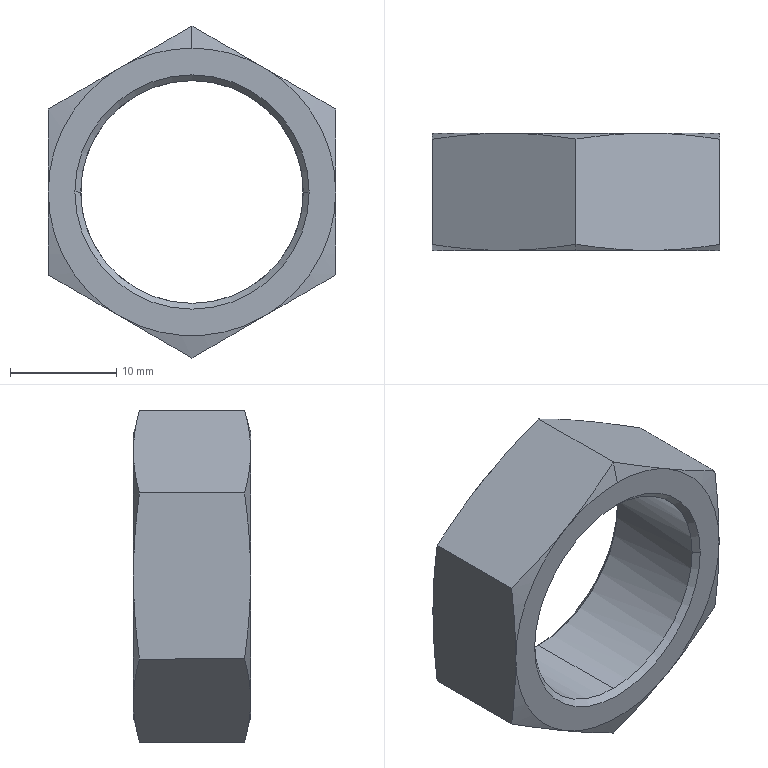Part | STEP file | 3 | 1 solid | 27 faces | box 27 x 11 x 31.177 mm | volume 3125 mm3 | cone 17 | plane 8 | cylinder 2 | commonest cylinder face diameters 20.917 x2
STEP:
#1=CARTESIAN_POINT('',(0.,10.541,-10.459));
#2=VERTEX_POINT('',#1);
#3=CARTESIAN_POINT('',(-10.459,10.541,0.));
#4=VERTEX_POINT('',#3);
#5=CARTESIAN_POINT('',(0.,10.541,0.));
#6=DIRECTION('',(0.,1.,0.));
#7=DIRECTION('',(0.,0.,1.));
#8=AXIS2_PLACEMENT_3D('',#5,#6,#7);
#9=CIRCLE('',#8,10.459);
#10=EDGE_CURVE('',#2,#4,#9,.T.);
#11=ORIENTED_EDGE('',*,*,#10,.F.);
#12=CARTESIAN_POINT('',(0.,20.459,-10.459));
#13=VERTEX_POINT('',#12);
#14=CARTESIAN_POINT('',(0.,15.5,-10.459));
#15=DIRECTION('',(0.,1.,0.));
#16=VECTOR('',#15,1000.);
#17=LINE('',#14,#16);
#18=EDGE_CURVE('',#2,#13,#17,.T.);
#19=ORIENTED_EDGE('',*,*,#18,.T.);
#20=CARTESIAN_POINT('',(0.,20.459,10.459));
#21=VERTEX_POINT('',#20);
#22=CARTESIAN_POINT('',(0.,20.459,0.));
#23=DIRECTION('',(0.,-1.,0.));
#24=DIRECTION('',(0.,0.,1.));
#25=AXIS2_PLACEMENT_3D('',#22,#23,#24);
#26=CIRCLE('',#25,10.459);
#27=EDGE_CURVE('',#21,#13,#26,.T.);
#28=ORIENTED_EDGE('',*,*,#27,.F.);
#29=CARTESIAN_POINT('',(0.,10.541,10.459));
#30=VERTEX_POINT('',#29);
#31=CARTESIAN_POINT('',(0.,15.5,10.459));
#32=DIRECTION('',(0.,1.,0.));
#33=VECTOR('',#32,1000.);
#34=LINE('',#31,#33);
#35=EDGE_CURVE('',#30,#21,#34,.T.);
#36=ORIENTED_EDGE('',*,*,#35,.F.);
#37=CARTESIAN_POINT('',(0.,10.541,0.));
#38=DIRECTION('',(0.,1.,0.));
#39=DIRECTION('',(0.,0.,1.));
#40=AXIS2_PLACEMENT_3D('',#37,#38,#39);
#41=CIRCLE('',#40,10.459);
#42=EDGE_CURVE('',#4,#30,#41,.T.);
#43=ORIENTED_EDGE('',*,*,#42,.F.);
#44=EDGE_LOOP('',(#11,#19,#28,#36,#43));
#45=FACE_OUTER_BOUND('',#44,.T.);
#46=CARTESIAN_POINT('',(0.,15.5,0.));
#47=DIRECTION('',(0.,1.,0.));
#48=DIRECTION('',(0.,0.,1.));
#49=AXIS2_PLACEMENT_3D('',#46,#47,#48);
#50=CYLINDRICAL_SURFACE('',#49,10.459);
#51=ADVANCED_FACE('',(#45),#50,.F.);
#52=CARTESIAN_POINT('',(10.459,10.541,0.));
#53=VERTEX_POINT('',#52);
#54=CARTESIAN_POINT('',(0.,10.541,0.));
#55=DIRECTION('',(0.,1.,0.));
#56=DIRECTION('',(0.,0.,1.));
#57=AXIS2_PLACEMENT_3D('',#54,#55,#56);
#58=CIRCLE('',#57,10.459);
#59=EDGE_CURVE('',#53,#2,#58,.T.);
#60=ORIENTED_EDGE('',*,*,#59,.T.);
#61=ORIENTED_EDGE('',*,*,#10,.T.);
#62=CARTESIAN_POINT('',(-11.,10.,0.));
#63=VERTEX_POINT('',#62);
#64=CARTESIAN_POINT('',(-11.,10.,0.));
#65=DIRECTION('',(-0.7071,-0.7071,0.));
#66=VECTOR('',#65,1000.);
#67=LINE('',#64,#66);
#68=EDGE_CURVE('',#4,#63,#67,.T.);
#69=ORIENTED_EDGE('',*,*,#68,.T.);
#70=CARTESIAN_POINT('',(11.,10.,0.));
#71=VERTEX_POINT('',#70);
#72=CARTESIAN_POINT('',(0.,10.,0.));
#73=DIRECTION('',(0.,1.,0.));
#74=DIRECTION('',(1.,0.,0.));
#75=AXIS2_PLACEMENT_3D('',#72,#73,#74);
#76=CIRCLE('',#75,11.);
#77=EDGE_CURVE('',#71,#63,#76,.T.);
#78=ORIENTED_EDGE('',*,*,#77,.F.);
#79=CARTESIAN_POINT('',(11.,10.,0.));
#80=DIRECTION('',(0.7071,-0.7071,0.));
#81=VECTOR('',#80,1000.);
#82=LINE('',#79,#81);
#83=EDGE_CURVE('',#53,#71,#82,.T.);
#84=ORIENTED_EDGE('',*,*,#83,.F.);
#85=EDGE_LOOP('',(#60,#61,#69,#78,#84));
#86=FACE_OUTER_BOUND('',#85,.T.);
#87=CARTESIAN_POINT('',(0.,10.,0.));
#88=DIRECTION('',(0.,-1.,0.));
#89=DIRECTION('',(1.,0.,0.));
#90=AXIS2_PLACEMENT_3D('',#87,#88,#89);
#91=CONICAL_SURFACE('',#90,11.,0.7854);
#92=ADVANCED_FACE('',(#86),#91,.F.);
#93=ORIENTED_EDGE('',*,*,#27,.T.);
#94=CARTESIAN_POINT('',(0.,21.,-11.));
#95=VERTEX_POINT('',#94);
#96=CARTESIAN_POINT('',(0.,21.,-11.));
#97=DIRECTION('',(0.,0.7071,-0.7071));
#98=VECTOR('',#97,1000.);
#99=LINE('',#96,#98);
#100=EDGE_CURVE('',#13,#95,#99,.T.);
#101=ORIENTED_EDGE('',*,*,#100,.T.);
#102=CARTESIAN_POINT('',(0.,21.,11.));
#103=VERTEX_POINT('',#102);
#104=CARTESIAN_POINT('',(0.,21.,0.));
#105=DIRECTION('',(0.,-1.,0.));
#106=DIRECTION('',(0.,0.,1.));
#107=AXIS2_PLACEMENT_3D('',#104,#105,#106);
#108=CIRCLE('',#107,11.);
#109=EDGE_CURVE('',#103,#95,#108,.T.);
#110=ORIENTED_EDGE('',*,*,#109,.F.);
#111=CARTESIAN_POINT('',(0.,21.,11.));
#112=DIRECTION('',(0.,0.7071,0.7071));
#113=VECTOR('',#112,1000.);
#114=LINE('',#111,#113);
#115=EDGE_CURVE('',#21,#103,#114,.T.);
#116=ORIENTED_EDGE('',*,*,#115,.F.);
#117=EDGE_LOOP('',(#93,#101,#110,#116));
#118=FACE_OUTER_BOUND('',#117,.T.);
#119=CARTESIAN_POINT('',(0.,21.,0.));
#120=DIRECTION('',(0.,1.,0.));
#121=DIRECTION('',(0.,0.,1.));
#122=AXIS2_PLACEMENT_3D('',#119,#120,#121);
#123=CONICAL_SURFACE('',#122,11.,0.7854);
#124=ADVANCED_FACE('',(#118),#123,.F.);
#125=CARTESIAN_POINT('',(0.,10.,13.5));
#126=VERTEX_POINT('',#125);
#127=CARTESIAN_POINT('',(-6.75,10.,11.691));
#128=VERTEX_POINT('',#127);
#129=CARTESIAN_POINT('',(0.,10.,0.));
#130=DIRECTION('',(0.,-1.,0.));
#131=DIRECTION('',(0.,0.,1.));
#132=AXIS2_PLACEMENT_3D('',#129,#130,#131);
#133=CIRCLE('',#132,13.5);
#134=EDGE_CURVE('',#126,#128,#133,.T.);
#135=ORIENTED_EDGE('',*,*,#134,.F.);
#136=CARTESIAN_POINT('',(0.,10.56,15.588));
#137=VERTEX_POINT('',#136);
#138=CARTESIAN_POINT('',(0.,10.563,15.601));
#139=DIRECTION('',(0.,0.2588,0.9659));
#140=VECTOR('',#139,1000.);
#141=LINE('',#138,#140);
#142=EDGE_CURVE('',#126,#137,#141,.T.);
#143=ORIENTED_EDGE('',*,*,#142,.T.);
#144=CARTESIAN_POINT('',(0.,10.56,15.588));
#145=CARTESIAN_POINT('',(-1.12,10.386,14.942));
#146=CARTESIAN_POINT('',(-2.242,10.245,14.294));
#147=CARTESIAN_POINT('',(-4.492,10.052,12.995));
#148=CARTESIAN_POINT('',(-5.619,10.,12.344));
#149=CARTESIAN_POINT('',(-6.75,10.,11.691));
#150=B_SPLINE_CURVE_WITH_KNOTS('',3,(#144,#145,#146,#147,#148,#149),.UNSPECIFIED.,.F.,.F.,(4,2,4),(0.,0.003907,0.007814),.UNSPECIFIED.);
#151=EDGE_CURVE('',#137,#128,#150,.T.);
#152=ORIENTED_EDGE('',*,*,#151,.T.);
#153=EDGE_LOOP('',(#135,#143,#152));
#154=FACE_OUTER_BOUND('',#153,.T.);
#155=CARTESIAN_POINT('',(0.,10.563,0.));
#156=DIRECTION('',(0.,1.,0.));
#157=DIRECTION('',(0.,0.,1.));
#158=AXIS2_PLACEMENT_3D('',#155,#156,#157);
#159=CONICAL_SURFACE('',#158,15.601,1.309);
#160=ADVANCED_FACE('',(#154),#159,.T.);
#161=ORIENTED_EDGE('',*,*,#18,.F.);
#162=ORIENTED_EDGE('',*,*,#59,.F.);
#163=CARTESIAN_POINT('',(0.,10.541,0.));
#164=DIRECTION('',(0.,1.,0.));
#165=DIRECTION('',(0.,0.,1.));
#166=AXIS2_PLACEMENT_3D('',#163,#164,#165);
#167=CIRCLE('',#166,10.459);
#168=EDGE_CURVE('',#30,#53,#167,.T.);
#169=ORIENTED_EDGE('',*,*,#168,.F.);
#170=ORIENTED_EDGE('',*,*,#35,.T.);
#171=CARTESIAN_POINT('',(0.,20.459,0.));
#172=DIRECTION('',(0.,-1.,0.));
#173=DIRECTION('',(0.,0.,1.));
#174=AXIS2_PLACEMENT_3D('',#171,#172,#173);
#175=CIRCLE('',#174,10.459);
#176=EDGE_CURVE('',#13,#21,#175,.T.);
#177=ORIENTED_EDGE('',*,*,#176,.F.);
#178=EDGE_LOOP('',(#161,#162,#169,#170,#177));
#179=FACE_OUTER_BOUND('',#178,.T.);
#180=CARTESIAN_POINT('',(0.,15.5,0.));
#181=DIRECTION('',(0.,1.,0.));
#182=DIRECTION('',(0.,0.,1.));
#183=AXIS2_PLACEMENT_3D('',#180,#181,#182);
#184=CYLINDRICAL_SURFACE('',#183,10.459);
#185=ADVANCED_FACE('',(#179),#184,.F.);
#186=ORIENTED_EDGE('',*,*,#68,.F.);
#187=ORIENTED_EDGE('',*,*,#42,.T.);
#188=ORIENTED_EDGE('',*,*,#168,.T.);
#189=ORIENTED_EDGE('',*,*,#83,.T.);
#190=CARTESIAN_POINT('',(0.,10.,0.));
#191=DIRECTION('',(0.,1.,0.));
#192=DIRECTION('',(1.,0.,0.));
#193=AXIS2_PLACEMENT_3D('',#190,#191,#192);
#194=CIRCLE('',#193,11.);
#195=EDGE_CURVE('',#63,#71,#194,.T.);
#196=ORIENTED_EDGE('',*,*,#195,.F.);
#197=EDGE_LOOP('',(#186,#187,#188,#189,#196));
#198=FACE_OUTER_BOUND('',#197,.T.);
#199=CARTESIAN_POINT('',(0.,10.,0.));
#200=DIRECTION('',(0.,-1.,0.));
#201=DIRECTION('',(1.,0.,0.));
#202=AXIS2_PLACEMENT_3D('',#199,#200,#201);
#203=CONICAL_SURFACE('',#202,11.,0.7854);
#204=ADVANCED_FACE('',(#198),#203,.F.);
#205=ORIENTED_EDGE('',*,*,#100,.F.);
#206=ORIENTED_EDGE('',*,*,#176,.T.);
#207=ORIENTED_EDGE('',*,*,#115,.T.);
#208=CARTESIAN_POINT('',(0.,21.,0.));
#209=DIRECTION('',(0.,-1.,0.));
#210=DIRECTION('',(0.,0.,1.));
#211=AXIS2_PLACEMENT_3D('',#208,#209,#210);
#212=CIRCLE('',#211,11.);
#213=EDGE_CURVE('',#95,#103,#212,.T.);
#214=ORIENTED_EDGE('',*,*,#213,.F.);
#215=EDGE_LOOP('',(#205,#206,#207,#214));
#216=FACE_OUTER_BOUND('',#215,.T.);
#217=CARTESIAN_POINT('',(0.,21.,0.));
#218=DIRECTION('',(0.,1.,0.));
#219=DIRECTION('',(0.,0.,1.));
#220=AXIS2_PLACEMENT_3D('',#217,#218,#219);
#221=CONICAL_SURFACE('',#220,11.,0.7854);
#222=ADVANCED_FACE('',(#216),#221,.F.);
#223=CARTESIAN_POINT('',(-13.5,10.,0.));
#224=VERTEX_POINT('',#223);
#225=CARTESIAN_POINT('',(0.,10.,0.));
#226=DIRECTION('',(0.,-1.,0.));
#227=DIRECTION('',(0.,0.,1.));
#228=AXIS2_PLACEMENT_3D('',#225,#226,#227);
#229=CIRCLE('',#228,13.5);
#230=EDGE_CURVE('',#128,#224,#229,.T.);
#231=ORIENTED_EDGE('',*,*,#230,.T.);
#232=CARTESIAN_POINT('',(-6.75,10.,-11.691));
#233=VERTEX_POINT('',#232);
#234=CARTESIAN_POINT('',(0.,10.,0.));
#235=DIRECTION('',(0.,-1.,0.));
#236=DIRECTION('',(0.,0.,1.));
#237=AXIS2_PLACEMENT_3D('',#234,#235,#236);
#238=CIRCLE('',#237,13.5);
#239=EDGE_CURVE('',#224,#233,#238,.T.);
#240=ORIENTED_EDGE('',*,*,#239,.T.);
#241=CARTESIAN_POINT('',(6.75,10.,-11.691));
#242=VERTEX_POINT('',#241);
#243=CARTESIAN_POINT('',(0.,10.,0.));
#244=DIRECTION('',(0.,-1.,0.));
#245=DIRECTION('',(0.,0.,1.));
#246=AXIS2_PLACEMENT_3D('',#243,#244,#245);
#247=CIRCLE('',#246,13.5);
#248=EDGE_CURVE('',#233,#242,#247,.T.);
#249=ORIENTED_EDGE('',*,*,#248,.T.);
#250=CARTESIAN_POINT('',(13.5,10.,0.));
#251=VERTEX_POINT('',#250);
#252=CARTESIAN_POINT('',(0.,10.,0.));
#253=DIRECTION('',(0.,-1.,0.));
#254=DIRECTION('',(0.,0.,1.));
#255=AXIS2_PLACEMENT_3D('',#252,#253,#254);
#256=CIRCLE('',#255,13.5);
#257=EDGE_CURVE('',#242,#251,#256,.T.);
#258=ORIENTED_EDGE('',*,*,#257,.T.);
#259=CARTESIAN_POINT('',(6.75,10.,11.691));
#260=VERTEX_POINT('',#259);
#261=CARTESIAN_POINT('',(0.,10.,0.));
#262=DIRECTION('',(0.,-1.,0.));
#263=DIRECTION('',(0.,0.,1.));
#264=AXIS2_PLACEMENT_3D('',#261,#262,#263);
#265=CIRCLE('',#264,13.5);
#266=EDGE_CURVE('',#251,#260,#265,.T.);
#267=ORIENTED_EDGE('',*,*,#266,.T.);
#268=CARTESIAN_POINT('',(0.,10.,0.));
#269=DIRECTION('',(0.,-1.,0.));
#270=DIRECTION('',(0.,0.,1.));
#271=AXIS2_PLACEMENT_3D('',#268,#269,#270);
#272=CIRCLE('',#271,13.5);
#273=EDGE_CURVE('',#260,#126,#272,.T.);
#274=ORIENTED_EDGE('',*,*,#273,.T.);
#275=ORIENTED_EDGE('',*,*,#134,.T.);
#276=EDGE_LOOP('',(#231,#240,#249,#258,#267,#274,#275));
#277=FACE_OUTER_BOUND('',#276,.T.);
#278=ORIENTED_EDGE('',*,*,#77,.T.);
#279=ORIENTED_EDGE('',*,*,#195,.T.);
#280=EDGE_LOOP('',(#278,#279));
#281=FACE_BOUND('',#280,.T.);
#282=CARTESIAN_POINT('',(0.,10.,-6.75));
#283=DIRECTION('',(0.,-1.,0.));
#284=DIRECTION('',(0.,0.,-1.));
#285=AXIS2_PLACEMENT_3D('',#282,#283,#284);
#286=PLANE('',#285);
#287=ADVANCED_FACE('',(#277,#281),#286,.T.);
#288=CARTESIAN_POINT('',(13.5,21.,0.));
#289=VERTEX_POINT('',#288);
#290=CARTESIAN_POINT('',(6.75,21.,-11.691));
#291=VERTEX_POINT('',#290);
#292=CARTESIAN_POINT('',(0.,21.,0.));
#293=DIRECTION('',(0.,1.,0.));
#294=DIRECTION('',(0.,0.,-1.));
#295=AXIS2_PLACEMENT_3D('',#292,#293,#294);
#296=CIRCLE('',#295,13.5);
#297=EDGE_CURVE('',#289,#291,#296,.T.);
#298=ORIENTED_EDGE('',*,*,#297,.T.);
#299=CARTESIAN_POINT('',(-6.75,21.,-11.691));
#300=VERTEX_POINT('',#299);
#301=CARTESIAN_POINT('',(0.,21.,0.));
#302=DIRECTION('',(0.,1.,0.));
#303=DIRECTION('',(1.,0.,0.));
#304=AXIS2_PLACEMENT_3D('',#301,#302,#303);
#305=CIRCLE('',#304,13.5);
#306=EDGE_CURVE('',#291,#300,#305,.T.);
#307=ORIENTED_EDGE('',*,*,#306,.T.);
#308=CARTESIAN_POINT('',(-13.5,21.,0.));
#309=VERTEX_POINT('',#308);
#310=CARTESIAN_POINT('',(0.,21.,0.));
#311=DIRECTION('',(0.,1.,0.));
#312=DIRECTION('',(0.,0.,-1.));
#313=AXIS2_PLACEMENT_3D('',#310,#311,#312);
#314=CIRCLE('',#313,13.5);
#315=EDGE_CURVE('',#300,#309,#314,.T.);
#316=ORIENTED_EDGE('',*,*,#315,.T.);
#317=CARTESIAN_POINT('',(-6.75,21.,11.691));
#318=VERTEX_POINT('',#317);
#319=CARTESIAN_POINT('',(0.,21.,0.));
#320=DIRECTION('',(0.,1.,0.));
#321=DIRECTION('',(0.,0.,-1.));
#322=AXIS2_PLACEMENT_3D('',#319,#320,#321);
#323=CIRCLE('',#322,13.5);
#324=EDGE_CURVE('',#309,#318,#323,.T.);
#325=ORIENTED_EDGE('',*,*,#324,.T.);
#326=CARTESIAN_POINT('',(6.75,21.,11.691));
#327=VERTEX_POINT('',#326);
#328=CARTESIAN_POINT('',(0.,21.,0.));
#329=DIRECTION('',(0.,1.,0.));
#330=DIRECTION('',(1.,0.,0.));
#331=AXIS2_PLACEMENT_3D('',#328,#329,#330);
#332=CIRCLE('',#331,13.5);
#333=EDGE_CURVE('',#318,#327,#332,.T.);
#334=ORIENTED_EDGE('',*,*,#333,.T.);
#335=CARTESIAN_POINT('',(0.,21.,0.));
#336=DIRECTION('',(0.,1.,0.));
#337=DIRECTION('',(0.,0.,-1.));
#338=AXIS2_PLACEMENT_3D('',#335,#336,#337);
#339=CIRCLE('',#338,13.5);
#340=EDGE_CURVE('',#327,#289,#339,.T.);
#341=ORIENTED_EDGE('',*,*,#340,.T.);
#342=EDGE_LOOP('',(#298,#307,#316,#325,#334,#341));
#343=FACE_OUTER_BOUND('',#342,.T.);
#344=ORIENTED_EDGE('',*,*,#109,.T.);
#345=ORIENTED_EDGE('',*,*,#213,.T.);
#346=EDGE_LOOP('',(#344,#345));
#347=FACE_BOUND('',#346,.T.);
#348=CARTESIAN_POINT('',(0.,21.,-6.75));
#349=DIRECTION('',(0.,1.,0.));
#350=DIRECTION('',(0.,0.,1.));
#351=AXIS2_PLACEMENT_3D('',#348,#349,#350);
#352=PLANE('',#351);
#353=ADVANCED_FACE('',(#343,#347),#352,.T.);
#354=CARTESIAN_POINT('',(-13.5,10.56,-7.794));
#355=VERTEX_POINT('',#354);
#356=CARTESIAN_POINT('',(-13.5,10.56,-7.794));
#357=CARTESIAN_POINT('',(-12.38,10.386,-8.441));
#358=CARTESIAN_POINT('',(-11.258,10.245,-9.089));
#359=CARTESIAN_POINT('',(-9.008,10.052,-10.387));
#360=CARTESIAN_POINT('',(-7.881,10.,-11.038));
#361=CARTESIAN_POINT('',(-6.75,10.,-11.691));
#362=B_SPLINE_CURVE_WITH_KNOTS('',3,(#356,#357,#358,#359,#360,#361),.UNSPECIFIED.,.F.,.F.,(4,2,4),(0.,0.003907,0.007814),.UNSPECIFIED.);
#363=EDGE_CURVE('',#355,#233,#362,.T.);
#364=ORIENTED_EDGE('',*,*,#363,.T.);
#365=ORIENTED_EDGE('',*,*,#239,.F.);
#366=CARTESIAN_POINT('',(-13.5,10.,0.));
#367=CARTESIAN_POINT('',(-13.5,10.,-1.306));
#368=CARTESIAN_POINT('',(-13.5,10.052,-2.608));
#369=CARTESIAN_POINT('',(-13.5,10.245,-5.205));
#370=CARTESIAN_POINT('',(-13.5,10.386,-6.501));
#371=CARTESIAN_POINT('',(-13.5,10.56,-7.794));
#372=B_SPLINE_CURVE_WITH_KNOTS('',3,(#366,#367,#368,#369,#370,#371),.UNSPECIFIED.,.F.,.F.,(4,2,4),(0.,0.003907,0.007814),.UNSPECIFIED.);
#373=EDGE_CURVE('',#224,#355,#372,.T.);
#374=ORIENTED_EDGE('',*,*,#373,.T.);
#375=EDGE_LOOP('',(#364,#365,#374));
#376=FACE_OUTER_BOUND('',#375,.T.);
#377=CARTESIAN_POINT('',(0.,10.563,0.));
#378=DIRECTION('',(0.,1.,0.));
#379=DIRECTION('',(0.,0.,1.));
#380=AXIS2_PLACEMENT_3D('',#377,#378,#379);
#381=CONICAL_SURFACE('',#380,15.601,1.309);
#382=ADVANCED_FACE('',(#376),#381,.T.);
#383=CARTESIAN_POINT('',(-13.5,10.56,7.794));
#384=VERTEX_POINT('',#383);
#385=CARTESIAN_POINT('',(-13.5,10.56,7.794));
#386=CARTESIAN_POINT('',(-13.5,10.386,6.501));
#387=CARTESIAN_POINT('',(-13.5,10.245,5.205));
#388=CARTESIAN_POINT('',(-13.5,10.052,2.608));
#389=CARTESIAN_POINT('',(-13.5,10.,1.306));
#390=CARTESIAN_POINT('',(-13.5,10.,0.));
#391=B_SPLINE_CURVE_WITH_KNOTS('',3,(#385,#386,#387,#388,#389,#390),.UNSPECIFIED.,.F.,.F.,(4,2,4),(0.,0.003907,0.007814),.UNSPECIFIED.);
#392=EDGE_CURVE('',#384,#224,#391,.T.);
#393=ORIENTED_EDGE('',*,*,#392,.T.);
#394=ORIENTED_EDGE('',*,*,#230,.F.);
#395=CARTESIAN_POINT('',(-6.75,10.,11.691));
#396=CARTESIAN_POINT('',(-7.881,10.,11.038));
#397=CARTESIAN_POINT('',(-9.008,10.052,10.387));
#398=CARTESIAN_POINT('',(-11.258,10.245,9.089));
#399=CARTESIAN_POINT('',(-12.38,10.386,8.441));
#400=CARTESIAN_POINT('',(-13.5,10.56,7.794));
#401=B_SPLINE_CURVE_WITH_KNOTS('',3,(#395,#396,#397,#398,#399,#400),.UNSPECIFIED.,.F.,.F.,(4,2,4),(0.,0.003907,0.007814),.UNSPECIFIED.);
#402=EDGE_CURVE('',#128,#384,#401,.T.);
#403=ORIENTED_EDGE('',*,*,#402,.T.);
#404=EDGE_LOOP('',(#393,#394,#403));
#405=FACE_OUTER_BOUND('',#404,.T.);
#406=CARTESIAN_POINT('',(0.,10.563,0.));
#407=DIRECTION('',(0.,1.,0.));
#408=DIRECTION('',(0.,0.,1.));
#409=AXIS2_PLACEMENT_3D('',#406,#407,#408);
#410=CONICAL_SURFACE('',#409,15.601,1.309);
#411=ADVANCED_FACE('',(#405),#410,.T.);
#412=ORIENTED_EDGE('',*,*,#142,.F.);
#413=ORIENTED_EDGE('',*,*,#273,.F.);
#414=CARTESIAN_POINT('',(6.75,10.,11.691));
#415=CARTESIAN_POINT('',(5.619,10.,12.344));
#416=CARTESIAN_POINT('',(4.492,10.052,12.995));
#417=CARTESIAN_POINT('',(2.242,10.245,14.294));
#418=CARTESIAN_POINT('',(1.12,10.386,14.942));
#419=CARTESIAN_POINT('',(0.,10.56,15.588));
#420=B_SPLINE_CURVE_WITH_KNOTS('',3,(#414,#415,#416,#417,#418,#419),.UNSPECIFIED.,.F.,.F.,(4,2,4),(0.,0.003907,0.007814),.UNSPECIFIED.);
#421=EDGE_CURVE('',#260,#137,#420,.T.);
#422=ORIENTED_EDGE('',*,*,#421,.T.);
#423=EDGE_LOOP('',(#412,#413,#422));
#424=FACE_OUTER_BOUND('',#423,.T.);
#425=CARTESIAN_POINT('',(0.,10.563,0.));
#426=DIRECTION('',(0.,1.,0.));
#427=DIRECTION('',(0.,0.,1.));
#428=AXIS2_PLACEMENT_3D('',#425,#426,#427);
#429=CONICAL_SURFACE('',#428,15.601,1.309);
#430=ADVANCED_FACE('',(#424),#429,.T.);
#431=ORIENTED_EDGE('',*,*,#266,.F.);
#432=CARTESIAN_POINT('',(13.5,10.56,7.794));
#433=VERTEX_POINT('',#432);
#434=CARTESIAN_POINT('',(13.5,10.,0.));
#435=CARTESIAN_POINT('',(13.5,10.,1.306));
#436=CARTESIAN_POINT('',(13.5,10.052,2.608));
#437=CARTESIAN_POINT('',(13.5,10.245,5.205));
#438=CARTESIAN_POINT('',(13.5,10.386,6.501));
#439=CARTESIAN_POINT('',(13.5,10.56,7.794));
#440=B_SPLINE_CURVE_WITH_KNOTS('',3,(#434,#435,#436,#437,#438,#439),.UNSPECIFIED.,.F.,.F.,(4,2,4),(0.,0.003907,0.007814),.UNSPECIFIED.);
#441=EDGE_CURVE('',#251,#433,#440,.T.);
#442=ORIENTED_EDGE('',*,*,#441,.T.);
#443=CARTESIAN_POINT('',(13.5,10.56,7.794));
#444=CARTESIAN_POINT('',(12.38,10.386,8.441));
#445=CARTESIAN_POINT('',(11.258,10.245,9.089));
#446=CARTESIAN_POINT('',(9.008,10.052,10.387));
#447=CARTESIAN_POINT('',(7.881,10.,11.038));
#448=CARTESIAN_POINT('',(6.75,10.,11.691));
#449=B_SPLINE_CURVE_WITH_KNOTS('',3,(#443,#444,#445,#446,#447,#448),.UNSPECIFIED.,.F.,.F.,(4,2,4),(0.,0.003907,0.007814),.UNSPECIFIED.);
#450=EDGE_CURVE('',#433,#260,#449,.T.);
#451=ORIENTED_EDGE('',*,*,#450,.T.);
#452=EDGE_LOOP('',(#431,#442,#451));
#453=FACE_OUTER_BOUND('',#452,.T.);
#454=CARTESIAN_POINT('',(0.,10.563,0.));
#455=DIRECTION('',(0.,1.,0.));
#456=DIRECTION('',(0.,0.,1.));
#457=AXIS2_PLACEMENT_3D('',#454,#455,#456);
#458=CONICAL_SURFACE('',#457,15.601,1.309);
#459=ADVANCED_FACE('',(#453),#458,.T.);
#460=ORIENTED_EDGE('',*,*,#257,.F.);
#461=CARTESIAN_POINT('',(13.5,10.56,-7.794));
#462=VERTEX_POINT('',#461);
#463=CARTESIAN_POINT('',(6.75,10.,-11.691));
#464=CARTESIAN_POINT('',(7.881,10.,-11.038));
#465=CARTESIAN_POINT('',(9.008,10.052,-10.387));
#466=CARTESIAN_POINT('',(11.258,10.245,-9.089));
#467=CARTESIAN_POINT('',(12.38,10.386,-8.441));
#468=CARTESIAN_POINT('',(13.5,10.56,-7.794));
#469=B_SPLINE_CURVE_WITH_KNOTS('',3,(#463,#464,#465,#466,#467,#468),.UNSPECIFIED.,.F.,.F.,(4,2,4),(0.,0.003907,0.007814),.UNSPECIFIED.);
#470=EDGE_CURVE('',#242,#462,#469,.T.);
#471=ORIENTED_EDGE('',*,*,#470,.T.);
#472=CARTESIAN_POINT('',(13.5,10.56,-7.794));
#473=CARTESIAN_POINT('',(13.5,10.386,-6.501));
#474=CARTESIAN_POINT('',(13.5,10.245,-5.205));
#475=CARTESIAN_POINT('',(13.5,10.052,-2.608));
#476=CARTESIAN_POINT('',(13.5,10.,-1.306));
#477=CARTESIAN_POINT('',(13.5,10.,0.));
#478=B_SPLINE_CURVE_WITH_KNOTS('',3,(#472,#473,#474,#475,#476,#477),.UNSPECIFIED.,.F.,.F.,(4,2,4),(0.,0.003907,0.007814),.UNSPECIFIED.);
#479=EDGE_CURVE('',#462,#251,#478,.T.);
#480=ORIENTED_EDGE('',*,*,#479,.T.);
#481=EDGE_LOOP('',(#460,#471,#480));
#482=FACE_OUTER_BOUND('',#481,.T.);
#483=CARTESIAN_POINT('',(0.,10.563,0.));
#484=DIRECTION('',(0.,1.,0.));
#485=DIRECTION('',(0.,0.,1.));
#486=AXIS2_PLACEMENT_3D('',#483,#484,#485);
#487=CONICAL_SURFACE('',#486,15.601,1.309);
#488=ADVANCED_FACE('',(#482),#487,.T.);
#489=CARTESIAN_POINT('',(0.,10.56,-15.588));
#490=VERTEX_POINT('',#489);
#491=CARTESIAN_POINT('',(0.,10.56,-15.588));
#492=CARTESIAN_POINT('',(1.12,10.386,-14.942));
#493=CARTESIAN_POINT('',(2.242,10.245,-14.294));
#494=CARTESIAN_POINT('',(4.492,10.052,-12.995));
#495=CARTESIAN_POINT('',(5.619,10.,-12.344));
#496=CARTESIAN_POINT('',(6.75,10.,-11.691));
#497=B_SPLINE_CURVE_WITH_KNOTS('',3,(#491,#492,#493,#494,#495,#496),.UNSPECIFIED.,.F.,.F.,(4,2,4),(0.,0.003907,0.007814),.UNSPECIFIED.);
#498=EDGE_CURVE('',#490,#242,#497,.T.);
#499=ORIENTED_EDGE('',*,*,#498,.T.);
#500=ORIENTED_EDGE('',*,*,#248,.F.);
#501=CARTESIAN_POINT('',(-6.75,10.,-11.691));
#502=CARTESIAN_POINT('',(-5.619,10.,-12.344));
#503=CARTESIAN_POINT('',(-4.492,10.052,-12.995));
#504=CARTESIAN_POINT('',(-2.242,10.245,-14.294));
#505=CARTESIAN_POINT('',(-1.12,10.386,-14.942));
#506=CARTESIAN_POINT('',(0.,10.56,-15.588));
#507=B_SPLINE_CURVE_WITH_KNOTS('',3,(#501,#502,#503,#504,#505,#506),.UNSPECIFIED.,.F.,.F.,(4,2,4),(0.,0.003907,0.007814),.UNSPECIFIED.);
#508=EDGE_CURVE('',#233,#490,#507,.T.);
#509=ORIENTED_EDGE('',*,*,#508,.T.);
#510=EDGE_LOOP('',(#499,#500,#509));
#511=FACE_OUTER_BOUND('',#510,.T.);
#512=CARTESIAN_POINT('',(0.,10.563,0.));
#513=DIRECTION('',(0.,1.,0.));
#514=DIRECTION('',(0.,0.,1.));
#515=AXIS2_PLACEMENT_3D('',#512,#513,#514);
#516=CONICAL_SURFACE('',#515,15.601,1.309);
#517=ADVANCED_FACE('',(#511),#516,.T.);
#518=ORIENTED_EDGE('',*,*,#306,.F.);
#519=CARTESIAN_POINT('',(0.,20.44,-15.588));
#520=VERTEX_POINT('',#519);
#521=CARTESIAN_POINT('',(6.75,21.,-11.691));
#522=CARTESIAN_POINT('',(5.619,21.,-12.344));
#523=CARTESIAN_POINT('',(4.492,20.948,-12.995));
#524=CARTESIAN_POINT('',(2.242,20.755,-14.294));
#525=CARTESIAN_POINT('',(1.12,20.614,-14.942));
#526=CARTESIAN_POINT('',(0.,20.44,-15.588));
#527=B_SPLINE_CURVE_WITH_KNOTS('',3,(#521,#522,#523,#524,#525,#526),.UNSPECIFIED.,.F.,.F.,(4,2,4),(0.,0.003907,0.007814),.UNSPECIFIED.);
#528=EDGE_CURVE('',#291,#520,#527,.T.);
#529=ORIENTED_EDGE('',*,*,#528,.T.);
#530=CARTESIAN_POINT('',(0.,20.44,-15.588));
#531=CARTESIAN_POINT('',(-1.12,20.614,-14.942));
#532=CARTESIAN_POINT('',(-2.242,20.755,-14.294));
#533=CARTESIAN_POINT('',(-4.492,20.948,-12.995));
#534=CARTESIAN_POINT('',(-5.619,21.,-12.344));
#535=CARTESIAN_POINT('',(-6.75,21.,-11.691));
#536=B_SPLINE_CURVE_WITH_KNOTS('',3,(#530,#531,#532,#533,#534,#535),.UNSPECIFIED.,.F.,.F.,(4,2,4),(0.,0.003907,0.007814),.UNSPECIFIED.);
#537=EDGE_CURVE('',#520,#300,#536,.T.);
#538=ORIENTED_EDGE('',*,*,#537,.T.);
#539=EDGE_LOOP('',(#518,#529,#538));
#540=FACE_OUTER_BOUND('',#539,.T.);
#541=CARTESIAN_POINT('',(0.,20.437,0.));
#542=DIRECTION('',(0.,-1.,0.));
#543=DIRECTION('',(1.,0.,0.));
#544=AXIS2_PLACEMENT_3D('',#541,#542,#543);
#545=CONICAL_SURFACE('',#544,15.601,1.309);
#546=ADVANCED_FACE('',(#540),#545,.T.);
#547=CARTESIAN_POINT('',(13.5,20.44,-7.794));
#548=VERTEX_POINT('',#547);
#549=CARTESIAN_POINT('',(13.5,20.44,-7.794));
#550=CARTESIAN_POINT('',(12.38,20.614,-8.441));
#551=CARTESIAN_POINT('',(11.258,20.755,-9.089));
#552=CARTESIAN_POINT('',(9.008,20.948,-10.387));
#553=CARTESIAN_POINT('',(7.881,21.,-11.038));
#554=CARTESIAN_POINT('',(6.75,21.,-11.691));
#555=B_SPLINE_CURVE_WITH_KNOTS('',3,(#549,#550,#551,#552,#553,#554),.UNSPECIFIED.,.F.,.F.,(4,2,4),(0.,0.003907,0.007814),.UNSPECIFIED.);
#556=EDGE_CURVE('',#548,#291,#555,.T.);
#557=ORIENTED_EDGE('',*,*,#556,.T.);
#558=ORIENTED_EDGE('',*,*,#297,.F.);
#559=CARTESIAN_POINT('',(13.5,21.,0.));
#560=CARTESIAN_POINT('',(13.5,21.,-1.306));
#561=CARTESIAN_POINT('',(13.5,20.948,-2.608));
#562=CARTESIAN_POINT('',(13.5,20.755,-5.205));
#563=CARTESIAN_POINT('',(13.5,20.614,-6.501));
#564=CARTESIAN_POINT('',(13.5,20.44,-7.794));
#565=B_SPLINE_CURVE_WITH_KNOTS('',3,(#559,#560,#561,#562,#563,#564),.UNSPECIFIED.,.F.,.F.,(4,2,4),(0.,0.003907,0.007814),.UNSPECIFIED.);
#566=EDGE_CURVE('',#289,#548,#565,.T.);
#567=ORIENTED_EDGE('',*,*,#566,.T.);
#568=EDGE_LOOP('',(#557,#558,#567));
#569=FACE_OUTER_BOUND('',#568,.T.);
#570=CARTESIAN_POINT('',(0.,20.437,0.));
#571=DIRECTION('',(0.,-1.,0.));
#572=DIRECTION('',(0.,0.,-1.));
#573=AXIS2_PLACEMENT_3D('',#570,#571,#572);
#574=CONICAL_SURFACE('',#573,15.601,1.309);
#575=ADVANCED_FACE('',(#569),#574,.T.);
#576=ORIENTED_EDGE('',*,*,#340,.F.);
#577=CARTESIAN_POINT('',(13.5,20.44,7.794));
#578=VERTEX_POINT('',#577);
#579=CARTESIAN_POINT('',(6.75,21.,11.691));
#580=CARTESIAN_POINT('',(7.881,21.,11.038));
#581=CARTESIAN_POINT('',(9.008,20.948,10.387));
#582=CARTESIAN_POINT('',(11.258,20.755,9.089));
#583=CARTESIAN_POINT('',(12.38,20.614,8.441));
#584=CARTESIAN_POINT('',(13.5,20.44,7.794));
#585=B_SPLINE_CURVE_WITH_KNOTS('',3,(#579,#580,#581,#582,#583,#584),.UNSPECIFIED.,.F.,.F.,(4,2,4),(0.,0.003907,0.007814),.UNSPECIFIED.);
#586=EDGE_CURVE('',#327,#578,#585,.T.);
#587=ORIENTED_EDGE('',*,*,#586,.T.);
#588=CARTESIAN_POINT('',(13.5,20.44,7.794));
#589=CARTESIAN_POINT('',(13.5,20.614,6.501));
#590=CARTESIAN_POINT('',(13.5,20.755,5.205));
#591=CARTESIAN_POINT('',(13.5,20.948,2.608));
#592=CARTESIAN_POINT('',(13.5,21.,1.306));
#593=CARTESIAN_POINT('',(13.5,21.,0.));
#594=B_SPLINE_CURVE_WITH_KNOTS('',3,(#588,#589,#590,#591,#592,#593),.UNSPECIFIED.,.F.,.F.,(4,2,4),(0.,0.003907,0.007814),.UNSPECIFIED.);
#595=EDGE_CURVE('',#578,#289,#594,.T.);
#596=ORIENTED_EDGE('',*,*,#595,.T.);
#597=EDGE_LOOP('',(#576,#587,#596));
#598=FACE_OUTER_BOUND('',#597,.T.);
#599=CARTESIAN_POINT('',(0.,20.437,0.));
#600=DIRECTION('',(0.,-1.,0.));
#601=DIRECTION('',(0.,0.,-1.));
#602=AXIS2_PLACEMENT_3D('',#599,#600,#601);
#603=CONICAL_SURFACE('',#602,15.601,1.309);
#604=ADVANCED_FACE('',(#598),#603,.T.);
#605=CARTESIAN_POINT('',(0.,20.44,15.588));
#606=VERTEX_POINT('',#605);
#607=CARTESIAN_POINT('',(0.,20.44,15.588));
#608=CARTESIAN_POINT('',(1.12,20.614,14.942));
#609=CARTESIAN_POINT('',(2.242,20.755,14.294));
#610=CARTESIAN_POINT('',(4.492,20.948,12.995));
#611=CARTESIAN_POINT('',(5.619,21.,12.344));
#612=CARTESIAN_POINT('',(6.75,21.,11.691));
#613=B_SPLINE_CURVE_WITH_KNOTS('',3,(#607,#608,#609,#610,#611,#612),.UNSPECIFIED.,.F.,.F.,(4,2,4),(0.,0.003907,0.007814),.UNSPECIFIED.);
#614=EDGE_CURVE('',#606,#327,#613,.T.);
#615=ORIENTED_EDGE('',*,*,#614,.T.);
#616=ORIENTED_EDGE('',*,*,#333,.F.);
#617=CARTESIAN_POINT('',(-6.75,21.,11.691));
#618=CARTESIAN_POINT('',(-5.619,21.,12.344));
#619=CARTESIAN_POINT('',(-4.492,20.948,12.995));
#620=CARTESIAN_POINT('',(-2.242,20.755,14.294));
#621=CARTESIAN_POINT('',(-1.12,20.614,14.942));
#622=CARTESIAN_POINT('',(0.,20.44,15.588));
#623=B_SPLINE_CURVE_WITH_KNOTS('',3,(#617,#618,#619,#620,#621,#622),.UNSPECIFIED.,.F.,.F.,(4,2,4),(0.,0.003907,0.007814),.UNSPECIFIED.);
#624=EDGE_CURVE('',#318,#606,#623,.T.);
#625=ORIENTED_EDGE('',*,*,#624,.T.);
#626=EDGE_LOOP('',(#615,#616,#625));
#627=FACE_OUTER_BOUND('',#626,.T.);
#628=CARTESIAN_POINT('',(0.,20.437,0.));
#629=DIRECTION('',(0.,-1.,0.));
#630=DIRECTION('',(1.,0.,0.));
#631=AXIS2_PLACEMENT_3D('',#628,#629,#630);
#632=CONICAL_SURFACE('',#631,15.601,1.309);
#633=ADVANCED_FACE('',(#627),#632,.T.);
#634=ORIENTED_EDGE('',*,*,#324,.F.);
#635=CARTESIAN_POINT('',(-13.5,20.44,7.794));
#636=VERTEX_POINT('',#635);
#637=CARTESIAN_POINT('',(-13.5,21.,0.));
#638=CARTESIAN_POINT('',(-13.5,21.,1.306));
#639=CARTESIAN_POINT('',(-13.5,20.948,2.608));
#640=CARTESIAN_POINT('',(-13.5,20.755,5.205));
#641=CARTESIAN_POINT('',(-13.5,20.614,6.501));
#642=CARTESIAN_POINT('',(-13.5,20.44,7.794));
#643=B_SPLINE_CURVE_WITH_KNOTS('',3,(#637,#638,#639,#640,#641,#642),.UNSPECIFIED.,.F.,.F.,(4,2,4),(0.,0.003907,0.007814),.UNSPECIFIED.);
#644=EDGE_CURVE('',#309,#636,#643,.T.);
#645=ORIENTED_EDGE('',*,*,#644,.T.);
#646=CARTESIAN_POINT('',(-13.5,20.44,7.794));
#647=CARTESIAN_POINT('',(-12.38,20.614,8.441));
#648=CARTESIAN_POINT('',(-11.258,20.755,9.089));
#649=CARTESIAN_POINT('',(-9.008,20.948,10.387));
#650=CARTESIAN_POINT('',(-7.881,21.,11.038));
#651=CARTESIAN_POINT('',(-6.75,21.,11.691));
#652=B_SPLINE_CURVE_WITH_KNOTS('',3,(#646,#647,#648,#649,#650,#651),.UNSPECIFIED.,.F.,.F.,(4,2,4),(0.,0.003907,0.007814),.UNSPECIFIED.);
#653=EDGE_CURVE('',#636,#318,#652,.T.);
#654=ORIENTED_EDGE('',*,*,#653,.T.);
#655=EDGE_LOOP('',(#634,#645,#654));
#656=FACE_OUTER_BOUND('',#655,.T.);
#657=CARTESIAN_POINT('',(0.,20.437,0.));
#658=DIRECTION('',(0.,-1.,0.));
#659=DIRECTION('',(0.,0.,-1.));
#660=AXIS2_PLACEMENT_3D('',#657,#658,#659);
#661=CONICAL_SURFACE('',#660,15.601,1.309);
#662=ADVANCED_FACE('',(#656),#661,.T.);
#663=CARTESIAN_POINT('',(-13.5,20.44,-7.794));
#664=VERTEX_POINT('',#663);
#665=CARTESIAN_POINT('',(-13.5,20.44,-7.794));
#666=CARTESIAN_POINT('',(-13.5,20.614,-6.501));
#667=CARTESIAN_POINT('',(-13.5,20.755,-5.205));
#668=CARTESIAN_POINT('',(-13.5,20.948,-2.608));
#669=CARTESIAN_POINT('',(-13.5,21.,-1.306));
#670=CARTESIAN_POINT('',(-13.5,21.,0.));
#671=B_SPLINE_CURVE_WITH_KNOTS('',3,(#665,#666,#667,#668,#669,#670),.UNSPECIFIED.,.F.,.F.,(4,2,4),(0.,0.003907,0.007814),.UNSPECIFIED.);
#672=EDGE_CURVE('',#664,#309,#671,.T.);
#673=ORIENTED_EDGE('',*,*,#672,.T.);
#674=ORIENTED_EDGE('',*,*,#315,.F.);
#675=CARTESIAN_POINT('',(-6.75,21.,-11.691));
#676=CARTESIAN_POINT('',(-7.881,21.,-11.038));
#677=CARTESIAN_POINT('',(-9.008,20.948,-10.387));
#678=CARTESIAN_POINT('',(-11.258,20.755,-9.089));
#679=CARTESIAN_POINT('',(-12.38,20.614,-8.441));
#680=CARTESIAN_POINT('',(-13.5,20.44,-7.794));
#681=B_SPLINE_CURVE_WITH_KNOTS('',3,(#675,#676,#677,#678,#679,#680),.UNSPECIFIED.,.F.,.F.,(4,2,4),(0.,0.003907,0.007814),.UNSPECIFIED.);
#682=EDGE_CURVE('',#300,#664,#681,.T.);
#683=ORIENTED_EDGE('',*,*,#682,.T.);
#684=EDGE_LOOP('',(#673,#674,#683));
#685=FACE_OUTER_BOUND('',#684,.T.);
#686=CARTESIAN_POINT('',(0.,20.437,0.));
#687=DIRECTION('',(0.,-1.,0.));
#688=DIRECTION('',(0.,0.,-1.));
#689=AXIS2_PLACEMENT_3D('',#686,#687,#688);
#690=CONICAL_SURFACE('',#689,15.601,1.309);
#691=ADVANCED_FACE('',(#685),#690,.T.);
#692=CARTESIAN_POINT('',(0.,10.,-15.588));
#693=DIRECTION('',(0.,1.,0.));
#694=VECTOR('',#693,1000.);
#695=LINE('',#692,#694);
#696=EDGE_CURVE('',#490,#520,#695,.T.);
#697=ORIENTED_EDGE('',*,*,#696,.F.);
#698=ORIENTED_EDGE('',*,*,#508,.F.);
#699=ORIENTED_EDGE('',*,*,#363,.F.);
#700=CARTESIAN_POINT('',(-13.5,10.,-7.794));
#701=DIRECTION('',(0.,-1.,0.));
#702=VECTOR('',#701,1000.);
#703=LINE('',#700,#702);
#704=EDGE_CURVE('',#664,#355,#703,.T.);
#705=ORIENTED_EDGE('',*,*,#704,.F.);
#706=ORIENTED_EDGE('',*,*,#682,.F.);
#707=ORIENTED_EDGE('',*,*,#537,.F.);
#708=EDGE_LOOP('',(#697,#698,#699,#705,#706,#707));
#709=FACE_OUTER_BOUND('',#708,.T.);
#710=CARTESIAN_POINT('',(0.,10.,-15.588));
#711=DIRECTION('',(0.5,0.,0.866));
#712=DIRECTION('',(0.866,0.,-0.5));
#713=AXIS2_PLACEMENT_3D('',#710,#711,#712);
#714=PLANE('',#713);
#715=ADVANCED_FACE('',(#709),#714,.F.);
#716=ORIENTED_EDGE('',*,*,#672,.F.);
#717=ORIENTED_EDGE('',*,*,#704,.T.);
#718=ORIENTED_EDGE('',*,*,#373,.F.);
#719=ORIENTED_EDGE('',*,*,#392,.F.);
#720=CARTESIAN_POINT('',(-13.5,10.,7.794));
#721=DIRECTION('',(0.,-1.,0.));
#722=VECTOR('',#721,1000.);
#723=LINE('',#720,#722);
#724=EDGE_CURVE('',#636,#384,#723,.T.);
#725=ORIENTED_EDGE('',*,*,#724,.F.);
#726=ORIENTED_EDGE('',*,*,#644,.F.);
#727=EDGE_LOOP('',(#716,#717,#718,#719,#725,#726));
#728=FACE_OUTER_BOUND('',#727,.T.);
#729=CARTESIAN_POINT('',(-13.5,10.,-7.794));
#730=DIRECTION('',(1.,0.,0.));
#731=DIRECTION('',(0.,0.,-1.));
#732=AXIS2_PLACEMENT_3D('',#729,#730,#731);
#733=PLANE('',#732);
#734=ADVANCED_FACE('',(#728),#733,.F.);
#735=ORIENTED_EDGE('',*,*,#653,.F.);
#736=ORIENTED_EDGE('',*,*,#724,.T.);
#737=ORIENTED_EDGE('',*,*,#402,.F.);
#738=ORIENTED_EDGE('',*,*,#151,.F.);
#739=CARTESIAN_POINT('',(0.,10.,15.588));
#740=DIRECTION('',(0.,-1.,0.));
#741=VECTOR('',#740,1000.);
#742=LINE('',#739,#741);
#743=EDGE_CURVE('',#606,#137,#742,.T.);
#744=ORIENTED_EDGE('',*,*,#743,.F.);
#745=ORIENTED_EDGE('',*,*,#624,.F.);
#746=EDGE_LOOP('',(#735,#736,#737,#738,#744,#745));
#747=FACE_OUTER_BOUND('',#746,.T.);
#748=CARTESIAN_POINT('',(-13.5,10.,7.794));
#749=DIRECTION('',(0.5,0.,-0.866));
#750=DIRECTION('',(-0.866,0.,-0.5));
#751=AXIS2_PLACEMENT_3D('',#748,#749,#750);
#752=PLANE('',#751);
#753=ADVANCED_FACE('',(#747),#752,.F.);
#754=ORIENTED_EDGE('',*,*,#614,.F.);
#755=ORIENTED_EDGE('',*,*,#743,.T.);
#756=ORIENTED_EDGE('',*,*,#421,.F.);
#757=ORIENTED_EDGE('',*,*,#450,.F.);
#758=CARTESIAN_POINT('',(13.5,10.,7.794));
#759=DIRECTION('',(0.,-1.,0.));
#760=VECTOR('',#759,1000.);
#761=LINE('',#758,#760);
#762=EDGE_CURVE('',#578,#433,#761,.T.);
#763=ORIENTED_EDGE('',*,*,#762,.F.);
#764=ORIENTED_EDGE('',*,*,#586,.F.);
#765=EDGE_LOOP('',(#754,#755,#756,#757,#763,#764));
#766=FACE_OUTER_BOUND('',#765,.T.);
#767=CARTESIAN_POINT('',(0.,10.,15.588));
#768=DIRECTION('',(-0.5,0.,-0.866));
#769=DIRECTION('',(-0.866,0.,0.5));
#770=AXIS2_PLACEMENT_3D('',#767,#768,#769);
#771=PLANE('',#770);
#772=ADVANCED_FACE('',(#766),#771,.F.);
#773=ORIENTED_EDGE('',*,*,#762,.T.);
#774=ORIENTED_EDGE('',*,*,#441,.F.);
#775=ORIENTED_EDGE('',*,*,#479,.F.);
#776=CARTESIAN_POINT('',(13.5,10.,-7.794));
#777=DIRECTION('',(0.,-1.,0.));
#778=VECTOR('',#777,1000.);
#779=LINE('',#776,#778);
#780=EDGE_CURVE('',#548,#462,#779,.T.);
#781=ORIENTED_EDGE('',*,*,#780,.F.);
#782=ORIENTED_EDGE('',*,*,#566,.F.);
#783=ORIENTED_EDGE('',*,*,#595,.F.);
#784=EDGE_LOOP('',(#773,#774,#775,#781,#782,#783));
#785=FACE_OUTER_BOUND('',#784,.T.);
#786=CARTESIAN_POINT('',(13.5,10.,7.794));
#787=DIRECTION('',(-1.,0.,0.));
#788=DIRECTION('',(0.,0.,1.));
#789=AXIS2_PLACEMENT_3D('',#786,#787,#788);
#790=PLANE('',#789);
#791=ADVANCED_FACE('',(#785),#790,.F.);
#792=ORIENTED_EDGE('',*,*,#780,.T.);
#793=ORIENTED_EDGE('',*,*,#470,.F.);
#794=ORIENTED_EDGE('',*,*,#498,.F.);
#795=ORIENTED_EDGE('',*,*,#696,.T.);
#796=ORIENTED_EDGE('',*,*,#528,.F.);
#797=ORIENTED_EDGE('',*,*,#556,.F.);
#798=EDGE_LOOP('',(#792,#793,#794,#795,#796,#797));
#799=FACE_OUTER_BOUND('',#798,.T.);
#800=CARTESIAN_POINT('',(13.5,10.,-7.794));
#801=DIRECTION('',(-0.5,0.,0.866));
#802=DIRECTION('',(0.866,0.,0.5));
#803=AXIS2_PLACEMENT_3D('',#800,#801,#802);
#804=PLANE('',#803);
#805=ADVANCED_FACE('',(#799),#804,.F.);
#806=CLOSED_SHELL('',(#51,#92,#124,#160,#185,#204,#222,#287,#353,#382,#411,#430,#459,#488,#517,#546,#575,#604,#633,#662,#691,#715,#734,#753,#772,#791,#805));
#807=MANIFOLD_SOLID_BREP('',#806);
#808=CARTESIAN_POINT('',(0.,0.,0.));
#809=DIRECTION('',(0.,0.,1.));
#810=DIRECTION('',(1.,0.,0.));
#811=AXIS2_PLACEMENT_3D('',#808,#809,#810);
#812=(LENGTH_UNIT()NAMED_UNIT(*)SI_UNIT(.MILLI.,.METRE.));
#813=UNCERTAINTY_MEASURE_WITH_UNIT(LENGTH_MEASURE(0.00001),#812,'','');
#814=(NAMED_UNIT(*)PLANE_ANGLE_UNIT()SI_UNIT($,.RADIAN.));
#815=(NAMED_UNIT(*)SI_UNIT($,.STERADIAN.)SOLID_ANGLE_UNIT());
#816=(GEOMETRIC_REPRESENTATION_CONTEXT(3)GLOBAL_UNCERTAINTY_ASSIGNED_CONTEXT((#813))GLOBAL_UNIT_ASSIGNED_CONTEXT((#812,#814,#815))REPRESENTATION_CONTEXT('',''));
#817=ADVANCED_BREP_SHAPE_REPRESENTATION('',(#807,#811),#816);